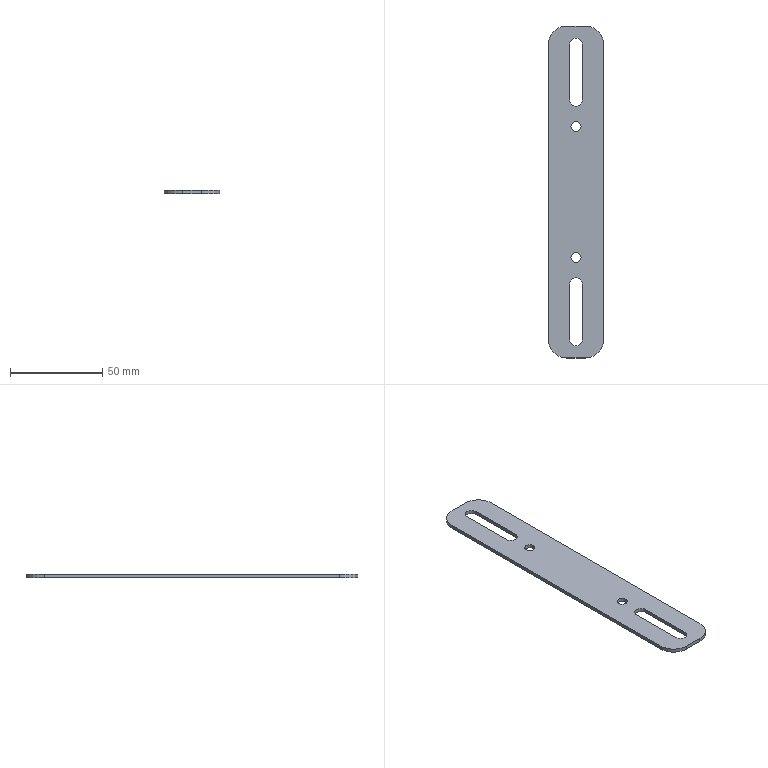Part | SolidWorks | features ICE 2, Extrusion 1, Fillet 1, MirrorPattern 1 | 1 solid | 22 faces | box 30 x 180 x 2 mm | volume 9539 mm3 | cylinder 12 | plane 10 | commonest cylinder face diameters 5.5 x4 7 x4 20 x4
STEP:
#1=CARTESIAN_POINT('',(-2.75,35.5,0.));
#2=VERTEX_POINT('',#1);
#3=CARTESIAN_POINT('',(2.75,35.5,0.));
#4=VERTEX_POINT('',#3);
#5=CARTESIAN_POINT('',(0.,35.5,0.));
#6=DIRECTION('',(0.,0.,1.));
#7=DIRECTION('',(1.,0.,0.));
#8=AXIS2_PLACEMENT_3D('',#5,#6,#7);
#9=CIRCLE('',#8,2.75);
#10=EDGE_CURVE('',#2,#4,#9,.T.);
#11=ORIENTED_EDGE('',*,*,#10,.F.);
#12=CARTESIAN_POINT('',(-2.75,35.5,2.));
#13=VERTEX_POINT('',#12);
#14=CARTESIAN_POINT('',(-2.75,35.5,0.));
#15=DIRECTION('',(0.,0.,1.));
#16=VECTOR('',#15,1000.);
#17=LINE('',#14,#16);
#18=EDGE_CURVE('',#2,#13,#17,.T.);
#19=ORIENTED_EDGE('',*,*,#18,.T.);
#20=CARTESIAN_POINT('',(2.75,35.5,2.));
#21=VERTEX_POINT('',#20);
#22=CARTESIAN_POINT('',(0.,35.5,2.));
#23=DIRECTION('',(0.,0.,1.));
#24=DIRECTION('',(1.,0.,0.));
#25=AXIS2_PLACEMENT_3D('',#22,#23,#24);
#26=CIRCLE('',#25,2.75);
#27=EDGE_CURVE('',#13,#21,#26,.T.);
#28=ORIENTED_EDGE('',*,*,#27,.T.);
#29=CARTESIAN_POINT('',(2.75,35.5,0.));
#30=DIRECTION('',(0.,0.,1.));
#31=VECTOR('',#30,1000.);
#32=LINE('',#29,#31);
#33=EDGE_CURVE('',#4,#21,#32,.T.);
#34=ORIENTED_EDGE('',*,*,#33,.F.);
#35=EDGE_LOOP('',(#11,#19,#28,#34));
#36=FACE_OUTER_BOUND('',#35,.T.);
#37=CARTESIAN_POINT('',(0.,35.5,0.));
#38=DIRECTION('',(0.,0.,1.));
#39=DIRECTION('',(1.,0.,0.));
#40=AXIS2_PLACEMENT_3D('',#37,#38,#39);
#41=CYLINDRICAL_SURFACE('',#40,2.75);
#42=ADVANCED_FACE('',(#36),#41,.F.);
#43=CARTESIAN_POINT('',(-2.75,-35.5,0.));
#44=VERTEX_POINT('',#43);
#45=CARTESIAN_POINT('',(2.75,-35.5,0.));
#46=VERTEX_POINT('',#45);
#47=CARTESIAN_POINT('',(0.,-35.5,0.));
#48=DIRECTION('',(0.,0.,1.));
#49=DIRECTION('',(1.,0.,0.));
#50=AXIS2_PLACEMENT_3D('',#47,#48,#49);
#51=CIRCLE('',#50,2.75);
#52=EDGE_CURVE('',#44,#46,#51,.T.);
#53=ORIENTED_EDGE('',*,*,#52,.F.);
#54=CARTESIAN_POINT('',(-2.75,-35.5,2.));
#55=VERTEX_POINT('',#54);
#56=CARTESIAN_POINT('',(-2.75,-35.5,0.));
#57=DIRECTION('',(0.,0.,1.));
#58=VECTOR('',#57,1000.);
#59=LINE('',#56,#58);
#60=EDGE_CURVE('',#44,#55,#59,.T.);
#61=ORIENTED_EDGE('',*,*,#60,.T.);
#62=CARTESIAN_POINT('',(2.75,-35.5,2.));
#63=VERTEX_POINT('',#62);
#64=CARTESIAN_POINT('',(0.,-35.5,2.));
#65=DIRECTION('',(0.,0.,1.));
#66=DIRECTION('',(1.,0.,0.));
#67=AXIS2_PLACEMENT_3D('',#64,#65,#66);
#68=CIRCLE('',#67,2.75);
#69=EDGE_CURVE('',#55,#63,#68,.T.);
#70=ORIENTED_EDGE('',*,*,#69,.T.);
#71=CARTESIAN_POINT('',(2.75,-35.5,0.));
#72=DIRECTION('',(0.,0.,1.));
#73=VECTOR('',#72,1000.);
#74=LINE('',#71,#73);
#75=EDGE_CURVE('',#46,#63,#74,.T.);
#76=ORIENTED_EDGE('',*,*,#75,.F.);
#77=EDGE_LOOP('',(#53,#61,#70,#76));
#78=FACE_OUTER_BOUND('',#77,.T.);
#79=CARTESIAN_POINT('',(0.,-35.5,0.));
#80=DIRECTION('',(0.,0.,1.));
#81=DIRECTION('',(1.,0.,0.));
#82=AXIS2_PLACEMENT_3D('',#79,#80,#81);
#83=CYLINDRICAL_SURFACE('',#82,2.75);
#84=ADVANCED_FACE('',(#78),#83,.F.);
#85=CARTESIAN_POINT('',(0.,35.5,2.));
#86=DIRECTION('',(0.,0.,1.));
#87=DIRECTION('',(1.,0.,0.));
#88=AXIS2_PLACEMENT_3D('',#85,#86,#87);
#89=CIRCLE('',#88,2.75);
#90=EDGE_CURVE('',#21,#13,#89,.T.);
#91=ORIENTED_EDGE('',*,*,#90,.F.);
#92=ORIENTED_EDGE('',*,*,#27,.F.);
#93=EDGE_LOOP('',(#91,#92));
#94=FACE_BOUND('',#93,.T.);
#95=CARTESIAN_POINT('',(0.,-35.5,2.));
#96=DIRECTION('',(0.,0.,1.));
#97=DIRECTION('',(1.,0.,0.));
#98=AXIS2_PLACEMENT_3D('',#95,#96,#97);
#99=CIRCLE('',#98,2.75);
#100=EDGE_CURVE('',#63,#55,#99,.T.);
#101=ORIENTED_EDGE('',*,*,#100,.F.);
#102=ORIENTED_EDGE('',*,*,#69,.F.);
#103=EDGE_LOOP('',(#101,#102));
#104=FACE_BOUND('',#103,.T.);
#105=CARTESIAN_POINT('',(-5.,-90.,2.));
#106=VERTEX_POINT('',#105);
#107=CARTESIAN_POINT('',(5.,-90.,2.));
#108=VERTEX_POINT('',#107);
#109=CARTESIAN_POINT('',(15.,-90.,2.));
#110=DIRECTION('',(1.,0.,0.));
#111=VECTOR('',#110,1000.);
#112=LINE('',#109,#111);
#113=EDGE_CURVE('',#106,#108,#112,.T.);
#114=ORIENTED_EDGE('',*,*,#113,.T.);
#115=CARTESIAN_POINT('',(15.,-80.,2.));
#116=VERTEX_POINT('',#115);
#117=CARTESIAN_POINT('',(5.,-80.,2.));
#118=DIRECTION('',(0.,0.,1.));
#119=DIRECTION('',(1.,0.,0.));
#120=AXIS2_PLACEMENT_3D('',#117,#118,#119);
#121=CIRCLE('',#120,10.);
#122=EDGE_CURVE('',#108,#116,#121,.T.);
#123=ORIENTED_EDGE('',*,*,#122,.T.);
#124=CARTESIAN_POINT('',(15.,80.,2.));
#125=VERTEX_POINT('',#124);
#126=CARTESIAN_POINT('',(15.,-90.,2.));
#127=DIRECTION('',(0.,1.,0.));
#128=VECTOR('',#127,1000.);
#129=LINE('',#126,#128);
#130=EDGE_CURVE('',#116,#125,#129,.T.);
#131=ORIENTED_EDGE('',*,*,#130,.T.);
#132=CARTESIAN_POINT('',(5.,90.,2.));
#133=VERTEX_POINT('',#132);
#134=CARTESIAN_POINT('',(5.,80.,2.));
#135=DIRECTION('',(0.,0.,1.));
#136=DIRECTION('',(1.,0.,0.));
#137=AXIS2_PLACEMENT_3D('',#134,#135,#136);
#138=CIRCLE('',#137,10.);
#139=EDGE_CURVE('',#125,#133,#138,.T.);
#140=ORIENTED_EDGE('',*,*,#139,.T.);
#141=CARTESIAN_POINT('',(-5.,90.,2.));
#142=VERTEX_POINT('',#141);
#143=CARTESIAN_POINT('',(15.,90.,2.));
#144=DIRECTION('',(-1.,0.,0.));
#145=VECTOR('',#144,1000.);
#146=LINE('',#143,#145);
#147=EDGE_CURVE('',#133,#142,#146,.T.);
#148=ORIENTED_EDGE('',*,*,#147,.T.);
#149=CARTESIAN_POINT('',(-15.,80.,2.));
#150=VERTEX_POINT('',#149);
#151=CARTESIAN_POINT('',(-5.,80.,2.));
#152=DIRECTION('',(0.,0.,1.));
#153=DIRECTION('',(1.,0.,0.));
#154=AXIS2_PLACEMENT_3D('',#151,#152,#153);
#155=CIRCLE('',#154,10.);
#156=EDGE_CURVE('',#142,#150,#155,.T.);
#157=ORIENTED_EDGE('',*,*,#156,.T.);
#158=CARTESIAN_POINT('',(-15.,-80.,2.));
#159=VERTEX_POINT('',#158);
#160=CARTESIAN_POINT('',(-15.,-90.,2.));
#161=DIRECTION('',(0.,-1.,0.));
#162=VECTOR('',#161,1000.);
#163=LINE('',#160,#162);
#164=EDGE_CURVE('',#150,#159,#163,.T.);
#165=ORIENTED_EDGE('',*,*,#164,.T.);
#166=CARTESIAN_POINT('',(-5.,-80.,2.));
#167=DIRECTION('',(0.,0.,1.));
#168=DIRECTION('',(1.,0.,0.));
#169=AXIS2_PLACEMENT_3D('',#166,#167,#168);
#170=CIRCLE('',#169,10.);
#171=EDGE_CURVE('',#159,#106,#170,.T.);
#172=ORIENTED_EDGE('',*,*,#171,.T.);
#173=EDGE_LOOP('',(#114,#123,#131,#140,#148,#157,#165,#172));
#174=FACE_OUTER_BOUND('',#173,.T.);
#175=CARTESIAN_POINT('',(3.5,80.,2.));
#176=VERTEX_POINT('',#175);
#177=CARTESIAN_POINT('',(-3.5,80.,2.));
#178=VERTEX_POINT('',#177);
#179=CARTESIAN_POINT('',(0.,80.,2.));
#180=DIRECTION('',(0.,0.,1.));
#181=DIRECTION('',(1.,0.,0.));
#182=AXIS2_PLACEMENT_3D('',#179,#180,#181);
#183=CIRCLE('',#182,3.5);
#184=EDGE_CURVE('',#176,#178,#183,.T.);
#185=ORIENTED_EDGE('',*,*,#184,.F.);
#186=CARTESIAN_POINT('',(3.5,50.,2.));
#187=VERTEX_POINT('',#186);
#188=CARTESIAN_POINT('',(3.5,80.,2.));
#189=DIRECTION('',(0.,1.,0.));
#190=VECTOR('',#189,1000.);
#191=LINE('',#188,#190);
#192=EDGE_CURVE('',#187,#176,#191,.T.);
#193=ORIENTED_EDGE('',*,*,#192,.F.);
#194=CARTESIAN_POINT('',(-3.5,50.,2.));
#195=VERTEX_POINT('',#194);
#196=CARTESIAN_POINT('',(0.,50.,2.));
#197=DIRECTION('',(0.,0.,1.));
#198=DIRECTION('',(1.,0.,0.));
#199=AXIS2_PLACEMENT_3D('',#196,#197,#198);
#200=CIRCLE('',#199,3.5);
#201=EDGE_CURVE('',#195,#187,#200,.T.);
#202=ORIENTED_EDGE('',*,*,#201,.F.);
#203=CARTESIAN_POINT('',(-3.5,80.,2.));
#204=DIRECTION('',(0.,-1.,0.));
#205=VECTOR('',#204,1000.);
#206=LINE('',#203,#205);
#207=EDGE_CURVE('',#178,#195,#206,.T.);
#208=ORIENTED_EDGE('',*,*,#207,.F.);
#209=EDGE_LOOP('',(#185,#193,#202,#208));
#210=FACE_BOUND('',#209,.T.);
#211=CARTESIAN_POINT('',(3.5,-50.,2.));
#212=VERTEX_POINT('',#211);
#213=CARTESIAN_POINT('',(3.5,-80.,2.));
#214=VERTEX_POINT('',#213);
#215=CARTESIAN_POINT('',(3.5,-80.,2.));
#216=DIRECTION('',(0.,-1.,0.));
#217=VECTOR('',#216,1000.);
#218=LINE('',#215,#217);
#219=EDGE_CURVE('',#212,#214,#218,.T.);
#220=ORIENTED_EDGE('',*,*,#219,.T.);
#221=CARTESIAN_POINT('',(-3.5,-80.,2.));
#222=VERTEX_POINT('',#221);
#223=CARTESIAN_POINT('',(0.,-80.,2.));
#224=DIRECTION('',(0.,0.,-1.));
#225=DIRECTION('',(1.,0.,0.));
#226=AXIS2_PLACEMENT_3D('',#223,#224,#225);
#227=CIRCLE('',#226,3.5);
#228=EDGE_CURVE('',#214,#222,#227,.T.);
#229=ORIENTED_EDGE('',*,*,#228,.T.);
#230=CARTESIAN_POINT('',(-3.5,-50.,2.));
#231=VERTEX_POINT('',#230);
#232=CARTESIAN_POINT('',(-3.5,-80.,2.));
#233=DIRECTION('',(0.,1.,0.));
#234=VECTOR('',#233,1000.);
#235=LINE('',#232,#234);
#236=EDGE_CURVE('',#222,#231,#235,.T.);
#237=ORIENTED_EDGE('',*,*,#236,.T.);
#238=CARTESIAN_POINT('',(0.,-50.,2.));
#239=DIRECTION('',(0.,0.,-1.));
#240=DIRECTION('',(1.,0.,0.));
#241=AXIS2_PLACEMENT_3D('',#238,#239,#240);
#242=CIRCLE('',#241,3.5);
#243=EDGE_CURVE('',#231,#212,#242,.T.);
#244=ORIENTED_EDGE('',*,*,#243,.T.);
#245=EDGE_LOOP('',(#220,#229,#237,#244));
#246=FACE_BOUND('',#245,.T.);
#247=CARTESIAN_POINT('',(0.,0.,2.));
#248=DIRECTION('',(0.,0.,1.));
#249=DIRECTION('',(1.,0.,0.));
#250=AXIS2_PLACEMENT_3D('',#247,#248,#249);
#251=PLANE('',#250);
#252=ADVANCED_FACE('',(#94,#104,#174,#210,#246),#251,.T.);
#253=CARTESIAN_POINT('',(0.,35.5,0.));
#254=DIRECTION('',(0.,0.,1.));
#255=DIRECTION('',(1.,0.,0.));
#256=AXIS2_PLACEMENT_3D('',#253,#254,#255);
#257=CIRCLE('',#256,2.75);
#258=EDGE_CURVE('',#4,#2,#257,.T.);
#259=ORIENTED_EDGE('',*,*,#258,.T.);
#260=ORIENTED_EDGE('',*,*,#10,.T.);
#261=EDGE_LOOP('',(#259,#260));
#262=FACE_BOUND('',#261,.T.);
#263=CARTESIAN_POINT('',(0.,-35.5,0.));
#264=DIRECTION('',(0.,0.,1.));
#265=DIRECTION('',(1.,0.,0.));
#266=AXIS2_PLACEMENT_3D('',#263,#264,#265);
#267=CIRCLE('',#266,2.75);
#268=EDGE_CURVE('',#46,#44,#267,.T.);
#269=ORIENTED_EDGE('',*,*,#268,.T.);
#270=ORIENTED_EDGE('',*,*,#52,.T.);
#271=EDGE_LOOP('',(#269,#270));
#272=FACE_BOUND('',#271,.T.);
#273=CARTESIAN_POINT('',(15.,-80.,0.));
#274=VERTEX_POINT('',#273);
#275=CARTESIAN_POINT('',(15.,80.,0.));
#276=VERTEX_POINT('',#275);
#277=CARTESIAN_POINT('',(15.,-90.,0.));
#278=DIRECTION('',(0.,1.,0.));
#279=VECTOR('',#278,1000.);
#280=LINE('',#277,#279);
#281=EDGE_CURVE('',#274,#276,#280,.T.);
#282=ORIENTED_EDGE('',*,*,#281,.F.);
#283=CARTESIAN_POINT('',(5.,-90.,0.));
#284=VERTEX_POINT('',#283);
#285=CARTESIAN_POINT('',(5.,-80.,0.));
#286=DIRECTION('',(0.,0.,-1.));
#287=DIRECTION('',(1.,0.,0.));
#288=AXIS2_PLACEMENT_3D('',#285,#286,#287);
#289=CIRCLE('',#288,10.);
#290=EDGE_CURVE('',#274,#284,#289,.T.);
#291=ORIENTED_EDGE('',*,*,#290,.T.);
#292=CARTESIAN_POINT('',(-5.,-90.,0.));
#293=VERTEX_POINT('',#292);
#294=CARTESIAN_POINT('',(15.,-90.,0.));
#295=DIRECTION('',(1.,0.,0.));
#296=VECTOR('',#295,1000.);
#297=LINE('',#294,#296);
#298=EDGE_CURVE('',#293,#284,#297,.T.);
#299=ORIENTED_EDGE('',*,*,#298,.F.);
#300=CARTESIAN_POINT('',(-15.,-80.,0.));
#301=VERTEX_POINT('',#300);
#302=CARTESIAN_POINT('',(-5.,-80.,0.));
#303=DIRECTION('',(0.,0.,-1.));
#304=DIRECTION('',(1.,0.,0.));
#305=AXIS2_PLACEMENT_3D('',#302,#303,#304);
#306=CIRCLE('',#305,10.);
#307=EDGE_CURVE('',#293,#301,#306,.T.);
#308=ORIENTED_EDGE('',*,*,#307,.T.);
#309=CARTESIAN_POINT('',(-15.,80.,0.));
#310=VERTEX_POINT('',#309);
#311=CARTESIAN_POINT('',(-15.,-90.,0.));
#312=DIRECTION('',(0.,-1.,0.));
#313=VECTOR('',#312,1000.);
#314=LINE('',#311,#313);
#315=EDGE_CURVE('',#310,#301,#314,.T.);
#316=ORIENTED_EDGE('',*,*,#315,.F.);
#317=CARTESIAN_POINT('',(-5.,90.,0.));
#318=VERTEX_POINT('',#317);
#319=CARTESIAN_POINT('',(-5.,80.,0.));
#320=DIRECTION('',(0.,0.,-1.));
#321=DIRECTION('',(1.,0.,0.));
#322=AXIS2_PLACEMENT_3D('',#319,#320,#321);
#323=CIRCLE('',#322,10.);
#324=EDGE_CURVE('',#310,#318,#323,.T.);
#325=ORIENTED_EDGE('',*,*,#324,.T.);
#326=CARTESIAN_POINT('',(5.,90.,0.));
#327=VERTEX_POINT('',#326);
#328=CARTESIAN_POINT('',(15.,90.,0.));
#329=DIRECTION('',(-1.,0.,0.));
#330=VECTOR('',#329,1000.);
#331=LINE('',#328,#330);
#332=EDGE_CURVE('',#327,#318,#331,.T.);
#333=ORIENTED_EDGE('',*,*,#332,.F.);
#334=CARTESIAN_POINT('',(5.,80.,0.));
#335=DIRECTION('',(0.,0.,-1.));
#336=DIRECTION('',(1.,0.,0.));
#337=AXIS2_PLACEMENT_3D('',#334,#335,#336);
#338=CIRCLE('',#337,10.);
#339=EDGE_CURVE('',#327,#276,#338,.T.);
#340=ORIENTED_EDGE('',*,*,#339,.T.);
#341=EDGE_LOOP('',(#282,#291,#299,#308,#316,#325,#333,#340));
#342=FACE_OUTER_BOUND('',#341,.T.);
#343=CARTESIAN_POINT('',(3.5,50.,0.));
#344=VERTEX_POINT('',#343);
#345=CARTESIAN_POINT('',(3.5,80.,0.));
#346=VERTEX_POINT('',#345);
#347=CARTESIAN_POINT('',(3.5,80.,0.));
#348=DIRECTION('',(0.,1.,0.));
#349=VECTOR('',#348,1000.);
#350=LINE('',#347,#349);
#351=EDGE_CURVE('',#344,#346,#350,.T.);
#352=ORIENTED_EDGE('',*,*,#351,.T.);
#353=CARTESIAN_POINT('',(-3.5,80.,0.));
#354=VERTEX_POINT('',#353);
#355=CARTESIAN_POINT('',(0.,80.,0.));
#356=DIRECTION('',(0.,0.,1.));
#357=DIRECTION('',(1.,0.,0.));
#358=AXIS2_PLACEMENT_3D('',#355,#356,#357);
#359=CIRCLE('',#358,3.5);
#360=EDGE_CURVE('',#346,#354,#359,.T.);
#361=ORIENTED_EDGE('',*,*,#360,.T.);
#362=CARTESIAN_POINT('',(-3.5,50.,0.));
#363=VERTEX_POINT('',#362);
#364=CARTESIAN_POINT('',(-3.5,80.,0.));
#365=DIRECTION('',(0.,-1.,0.));
#366=VECTOR('',#365,1000.);
#367=LINE('',#364,#366);
#368=EDGE_CURVE('',#354,#363,#367,.T.);
#369=ORIENTED_EDGE('',*,*,#368,.T.);
#370=CARTESIAN_POINT('',(0.,50.,0.));
#371=DIRECTION('',(0.,0.,1.));
#372=DIRECTION('',(1.,0.,0.));
#373=AXIS2_PLACEMENT_3D('',#370,#371,#372);
#374=CIRCLE('',#373,3.5);
#375=EDGE_CURVE('',#363,#344,#374,.T.);
#376=ORIENTED_EDGE('',*,*,#375,.T.);
#377=EDGE_LOOP('',(#352,#361,#369,#376));
#378=FACE_BOUND('',#377,.T.);
#379=CARTESIAN_POINT('',(3.5,-80.,0.));
#380=VERTEX_POINT('',#379);
#381=CARTESIAN_POINT('',(-3.5,-80.,0.));
#382=VERTEX_POINT('',#381);
#383=CARTESIAN_POINT('',(0.,-80.,0.));
#384=DIRECTION('',(0.,0.,-1.));
#385=DIRECTION('',(1.,0.,0.));
#386=AXIS2_PLACEMENT_3D('',#383,#384,#385);
#387=CIRCLE('',#386,3.5);
#388=EDGE_CURVE('',#380,#382,#387,.T.);
#389=ORIENTED_EDGE('',*,*,#388,.F.);
#390=CARTESIAN_POINT('',(3.5,-50.,0.));
#391=VERTEX_POINT('',#390);
#392=CARTESIAN_POINT('',(3.5,-80.,0.));
#393=DIRECTION('',(0.,-1.,0.));
#394=VECTOR('',#393,1000.);
#395=LINE('',#392,#394);
#396=EDGE_CURVE('',#391,#380,#395,.T.);
#397=ORIENTED_EDGE('',*,*,#396,.F.);
#398=CARTESIAN_POINT('',(-3.5,-50.,0.));
#399=VERTEX_POINT('',#398);
#400=CARTESIAN_POINT('',(0.,-50.,0.));
#401=DIRECTION('',(0.,0.,-1.));
#402=DIRECTION('',(1.,0.,0.));
#403=AXIS2_PLACEMENT_3D('',#400,#401,#402);
#404=CIRCLE('',#403,3.5);
#405=EDGE_CURVE('',#399,#391,#404,.T.);
#406=ORIENTED_EDGE('',*,*,#405,.F.);
#407=CARTESIAN_POINT('',(-3.5,-80.,0.));
#408=DIRECTION('',(0.,1.,0.));
#409=VECTOR('',#408,1000.);
#410=LINE('',#407,#409);
#411=EDGE_CURVE('',#382,#399,#410,.T.);
#412=ORIENTED_EDGE('',*,*,#411,.F.);
#413=EDGE_LOOP('',(#389,#397,#406,#412));
#414=FACE_BOUND('',#413,.T.);
#415=CARTESIAN_POINT('',(0.,0.,0.));
#416=DIRECTION('',(0.,0.,1.));
#417=DIRECTION('',(1.,0.,0.));
#418=AXIS2_PLACEMENT_3D('',#415,#416,#417);
#419=PLANE('',#418);
#420=ADVANCED_FACE('',(#262,#272,#342,#378,#414),#419,.F.);
#421=ORIENTED_EDGE('',*,*,#315,.T.);
#422=CARTESIAN_POINT('',(-15.,-80.,2.));
#423=DIRECTION('',(0.,0.,1.));
#424=VECTOR('',#423,1000.);
#425=LINE('',#422,#424);
#426=EDGE_CURVE('',#301,#159,#425,.T.);
#427=ORIENTED_EDGE('',*,*,#426,.T.);
#428=ORIENTED_EDGE('',*,*,#164,.F.);
#429=CARTESIAN_POINT('',(-15.,80.,2.));
#430=DIRECTION('',(0.,0.,-1.));
#431=VECTOR('',#430,1000.);
#432=LINE('',#429,#431);
#433=EDGE_CURVE('',#150,#310,#432,.T.);
#434=ORIENTED_EDGE('',*,*,#433,.T.);
#435=EDGE_LOOP('',(#421,#427,#428,#434));
#436=FACE_OUTER_BOUND('',#435,.T.);
#437=CARTESIAN_POINT('',(-15.,-90.,2.));
#438=DIRECTION('',(1.,0.,0.));
#439=DIRECTION('',(0.,0.,-1.));
#440=AXIS2_PLACEMENT_3D('',#437,#438,#439);
#441=PLANE('',#440);
#442=ADVANCED_FACE('',(#436),#441,.F.);
#443=ORIENTED_EDGE('',*,*,#298,.T.);
#444=CARTESIAN_POINT('',(5.,-90.,2.));
#445=DIRECTION('',(0.,0.,1.));
#446=VECTOR('',#445,1000.);
#447=LINE('',#444,#446);
#448=EDGE_CURVE('',#284,#108,#447,.T.);
#449=ORIENTED_EDGE('',*,*,#448,.T.);
#450=ORIENTED_EDGE('',*,*,#113,.F.);
#451=CARTESIAN_POINT('',(-5.,-90.,2.));
#452=DIRECTION('',(0.,0.,-1.));
#453=VECTOR('',#452,1000.);
#454=LINE('',#451,#453);
#455=EDGE_CURVE('',#106,#293,#454,.T.);
#456=ORIENTED_EDGE('',*,*,#455,.T.);
#457=EDGE_LOOP('',(#443,#449,#450,#456));
#458=FACE_OUTER_BOUND('',#457,.T.);
#459=CARTESIAN_POINT('',(15.,-90.,2.));
#460=DIRECTION('',(0.,1.,0.));
#461=DIRECTION('',(0.,0.,1.));
#462=AXIS2_PLACEMENT_3D('',#459,#460,#461);
#463=PLANE('',#462);
#464=ADVANCED_FACE('',(#458),#463,.F.);
#465=ORIENTED_EDGE('',*,*,#130,.F.);
#466=CARTESIAN_POINT('',(15.,-80.,2.));
#467=DIRECTION('',(0.,0.,-1.));
#468=VECTOR('',#467,1000.);
#469=LINE('',#466,#468);
#470=EDGE_CURVE('',#116,#274,#469,.T.);
#471=ORIENTED_EDGE('',*,*,#470,.T.);
#472=ORIENTED_EDGE('',*,*,#281,.T.);
#473=CARTESIAN_POINT('',(15.,80.,2.));
#474=DIRECTION('',(0.,0.,1.));
#475=VECTOR('',#474,1000.);
#476=LINE('',#473,#475);
#477=EDGE_CURVE('',#276,#125,#476,.T.);
#478=ORIENTED_EDGE('',*,*,#477,.T.);
#479=EDGE_LOOP('',(#465,#471,#472,#478));
#480=FACE_OUTER_BOUND('',#479,.T.);
#481=CARTESIAN_POINT('',(15.,-90.,2.));
#482=DIRECTION('',(-1.,0.,0.));
#483=DIRECTION('',(0.,0.,1.));
#484=AXIS2_PLACEMENT_3D('',#481,#482,#483);
#485=PLANE('',#484);
#486=ADVANCED_FACE('',(#480),#485,.F.);
#487=ORIENTED_EDGE('',*,*,#332,.T.);
#488=CARTESIAN_POINT('',(-5.,90.,2.));
#489=DIRECTION('',(0.,0.,1.));
#490=VECTOR('',#489,1000.);
#491=LINE('',#488,#490);
#492=EDGE_CURVE('',#318,#142,#491,.T.);
#493=ORIENTED_EDGE('',*,*,#492,.T.);
#494=ORIENTED_EDGE('',*,*,#147,.F.);
#495=CARTESIAN_POINT('',(5.,90.,2.));
#496=DIRECTION('',(0.,0.,-1.));
#497=VECTOR('',#496,1000.);
#498=LINE('',#495,#497);
#499=EDGE_CURVE('',#133,#327,#498,.T.);
#500=ORIENTED_EDGE('',*,*,#499,.T.);
#501=EDGE_LOOP('',(#487,#493,#494,#500));
#502=FACE_OUTER_BOUND('',#501,.T.);
#503=CARTESIAN_POINT('',(15.,90.,2.));
#504=DIRECTION('',(0.,-1.,0.));
#505=DIRECTION('',(0.,0.,-1.));
#506=AXIS2_PLACEMENT_3D('',#503,#504,#505);
#507=PLANE('',#506);
#508=ADVANCED_FACE('',(#502),#507,.F.);
#509=ORIENTED_EDGE('',*,*,#122,.F.);
#510=ORIENTED_EDGE('',*,*,#448,.F.);
#511=ORIENTED_EDGE('',*,*,#290,.F.);
#512=ORIENTED_EDGE('',*,*,#470,.F.);
#513=EDGE_LOOP('',(#509,#510,#511,#512));
#514=FACE_OUTER_BOUND('',#513,.T.);
#515=CARTESIAN_POINT('',(5.,-80.,2.));
#516=DIRECTION('',(0.,0.,-1.));
#517=DIRECTION('',(-1.,0.,0.));
#518=AXIS2_PLACEMENT_3D('',#515,#516,#517);
#519=CYLINDRICAL_SURFACE('',#518,10.);
#520=ADVANCED_FACE('',(#514),#519,.T.);
#521=ORIENTED_EDGE('',*,*,#171,.F.);
#522=ORIENTED_EDGE('',*,*,#426,.F.);
#523=ORIENTED_EDGE('',*,*,#307,.F.);
#524=ORIENTED_EDGE('',*,*,#455,.F.);
#525=EDGE_LOOP('',(#521,#522,#523,#524));
#526=FACE_OUTER_BOUND('',#525,.T.);
#527=CARTESIAN_POINT('',(-5.,-80.,2.));
#528=DIRECTION('',(0.,0.,-1.));
#529=DIRECTION('',(-1.,0.,0.));
#530=AXIS2_PLACEMENT_3D('',#527,#528,#529);
#531=CYLINDRICAL_SURFACE('',#530,10.);
#532=ADVANCED_FACE('',(#526),#531,.T.);
#533=ORIENTED_EDGE('',*,*,#156,.F.);
#534=ORIENTED_EDGE('',*,*,#492,.F.);
#535=ORIENTED_EDGE('',*,*,#324,.F.);
#536=ORIENTED_EDGE('',*,*,#433,.F.);
#537=EDGE_LOOP('',(#533,#534,#535,#536));
#538=FACE_OUTER_BOUND('',#537,.T.);
#539=CARTESIAN_POINT('',(-5.,80.,2.));
#540=DIRECTION('',(0.,0.,-1.));
#541=DIRECTION('',(-1.,0.,0.));
#542=AXIS2_PLACEMENT_3D('',#539,#540,#541);
#543=CYLINDRICAL_SURFACE('',#542,10.);
#544=ADVANCED_FACE('',(#538),#543,.T.);
#545=ORIENTED_EDGE('',*,*,#139,.F.);
#546=ORIENTED_EDGE('',*,*,#477,.F.);
#547=ORIENTED_EDGE('',*,*,#339,.F.);
#548=ORIENTED_EDGE('',*,*,#499,.F.);
#549=EDGE_LOOP('',(#545,#546,#547,#548));
#550=FACE_OUTER_BOUND('',#549,.T.);
#551=CARTESIAN_POINT('',(5.,80.,2.));
#552=DIRECTION('',(0.,0.,-1.));
#553=DIRECTION('',(-1.,0.,0.));
#554=AXIS2_PLACEMENT_3D('',#551,#552,#553);
#555=CYLINDRICAL_SURFACE('',#554,10.);
#556=ADVANCED_FACE('',(#550),#555,.T.);
#557=ORIENTED_EDGE('',*,*,#184,.T.);
#558=CARTESIAN_POINT('',(-3.5,80.,0.));
#559=DIRECTION('',(0.,0.,1.));
#560=VECTOR('',#559,1000.);
#561=LINE('',#558,#560);
#562=EDGE_CURVE('',#354,#178,#561,.T.);
#563=ORIENTED_EDGE('',*,*,#562,.F.);
#564=ORIENTED_EDGE('',*,*,#360,.F.);
#565=CARTESIAN_POINT('',(3.5,80.,0.));
#566=DIRECTION('',(0.,0.,1.));
#567=VECTOR('',#566,1000.);
#568=LINE('',#565,#567);
#569=EDGE_CURVE('',#346,#176,#568,.T.);
#570=ORIENTED_EDGE('',*,*,#569,.T.);
#571=EDGE_LOOP('',(#557,#563,#564,#570));
#572=FACE_OUTER_BOUND('',#571,.T.);
#573=CARTESIAN_POINT('',(0.,80.,0.));
#574=DIRECTION('',(0.,0.,1.));
#575=DIRECTION('',(1.,0.,0.));
#576=AXIS2_PLACEMENT_3D('',#573,#574,#575);
#577=CYLINDRICAL_SURFACE('',#576,3.5);
#578=ADVANCED_FACE('',(#572),#577,.F.);
#579=ORIENTED_EDGE('',*,*,#192,.T.);
#580=ORIENTED_EDGE('',*,*,#569,.F.);
#581=ORIENTED_EDGE('',*,*,#351,.F.);
#582=CARTESIAN_POINT('',(3.5,50.,0.));
#583=DIRECTION('',(0.,0.,1.));
#584=VECTOR('',#583,1000.);
#585=LINE('',#582,#584);
#586=EDGE_CURVE('',#344,#187,#585,.T.);
#587=ORIENTED_EDGE('',*,*,#586,.T.);
#588=EDGE_LOOP('',(#579,#580,#581,#587));
#589=FACE_OUTER_BOUND('',#588,.T.);
#590=CARTESIAN_POINT('',(3.5,80.,0.));
#591=DIRECTION('',(1.,0.,0.));
#592=DIRECTION('',(0.,1.,0.));
#593=AXIS2_PLACEMENT_3D('',#590,#591,#592);
#594=PLANE('',#593);
#595=ADVANCED_FACE('',(#589),#594,.F.);
#596=ORIENTED_EDGE('',*,*,#201,.T.);
#597=ORIENTED_EDGE('',*,*,#586,.F.);
#598=ORIENTED_EDGE('',*,*,#375,.F.);
#599=CARTESIAN_POINT('',(-3.5,50.,0.));
#600=DIRECTION('',(0.,0.,1.));
#601=VECTOR('',#600,1000.);
#602=LINE('',#599,#601);
#603=EDGE_CURVE('',#363,#195,#602,.T.);
#604=ORIENTED_EDGE('',*,*,#603,.T.);
#605=EDGE_LOOP('',(#596,#597,#598,#604));
#606=FACE_OUTER_BOUND('',#605,.T.);
#607=CARTESIAN_POINT('',(0.,50.,0.));
#608=DIRECTION('',(0.,0.,1.));
#609=DIRECTION('',(1.,0.,0.));
#610=AXIS2_PLACEMENT_3D('',#607,#608,#609);
#611=CYLINDRICAL_SURFACE('',#610,3.5);
#612=ADVANCED_FACE('',(#606),#611,.F.);
#613=ORIENTED_EDGE('',*,*,#207,.T.);
#614=ORIENTED_EDGE('',*,*,#603,.F.);
#615=ORIENTED_EDGE('',*,*,#368,.F.);
#616=ORIENTED_EDGE('',*,*,#562,.T.);
#617=EDGE_LOOP('',(#613,#614,#615,#616));
#618=FACE_OUTER_BOUND('',#617,.T.);
#619=CARTESIAN_POINT('',(-3.5,80.,0.));
#620=DIRECTION('',(-1.,0.,0.));
#621=DIRECTION('',(0.,-1.,0.));
#622=AXIS2_PLACEMENT_3D('',#619,#620,#621);
#623=PLANE('',#622);
#624=ADVANCED_FACE('',(#618),#623,.F.);
#625=ORIENTED_EDGE('',*,*,#228,.F.);
#626=CARTESIAN_POINT('',(3.5,-80.,0.));
#627=DIRECTION('',(0.,0.,1.));
#628=VECTOR('',#627,1000.);
#629=LINE('',#626,#628);
#630=EDGE_CURVE('',#380,#214,#629,.T.);
#631=ORIENTED_EDGE('',*,*,#630,.F.);
#632=ORIENTED_EDGE('',*,*,#388,.T.);
#633=CARTESIAN_POINT('',(-3.5,-80.,0.));
#634=DIRECTION('',(0.,0.,1.));
#635=VECTOR('',#634,1000.);
#636=LINE('',#633,#635);
#637=EDGE_CURVE('',#382,#222,#636,.T.);
#638=ORIENTED_EDGE('',*,*,#637,.T.);
#639=EDGE_LOOP('',(#625,#631,#632,#638));
#640=FACE_OUTER_BOUND('',#639,.T.);
#641=CARTESIAN_POINT('',(0.,-80.,0.));
#642=DIRECTION('',(0.,0.,1.));
#643=DIRECTION('',(1.,0.,0.));
#644=AXIS2_PLACEMENT_3D('',#641,#642,#643);
#645=CYLINDRICAL_SURFACE('',#644,3.5);
#646=ADVANCED_FACE('',(#640),#645,.F.);
#647=ORIENTED_EDGE('',*,*,#236,.F.);
#648=ORIENTED_EDGE('',*,*,#637,.F.);
#649=ORIENTED_EDGE('',*,*,#411,.T.);
#650=CARTESIAN_POINT('',(-3.5,-50.,0.));
#651=DIRECTION('',(0.,0.,1.));
#652=VECTOR('',#651,1000.);
#653=LINE('',#650,#652);
#654=EDGE_CURVE('',#399,#231,#653,.T.);
#655=ORIENTED_EDGE('',*,*,#654,.T.);
#656=EDGE_LOOP('',(#647,#648,#649,#655));
#657=FACE_OUTER_BOUND('',#656,.T.);
#658=CARTESIAN_POINT('',(-3.5,-80.,0.));
#659=DIRECTION('',(1.,0.,0.));
#660=DIRECTION('',(0.,1.,0.));
#661=AXIS2_PLACEMENT_3D('',#658,#659,#660);
#662=PLANE('',#661);
#663=ADVANCED_FACE('',(#657),#662,.T.);
#664=ORIENTED_EDGE('',*,*,#243,.F.);
#665=ORIENTED_EDGE('',*,*,#654,.F.);
#666=ORIENTED_EDGE('',*,*,#405,.T.);
#667=CARTESIAN_POINT('',(3.5,-50.,0.));
#668=DIRECTION('',(0.,0.,1.));
#669=VECTOR('',#668,1000.);
#670=LINE('',#667,#669);
#671=EDGE_CURVE('',#391,#212,#670,.T.);
#672=ORIENTED_EDGE('',*,*,#671,.T.);
#673=EDGE_LOOP('',(#664,#665,#666,#672));
#674=FACE_OUTER_BOUND('',#673,.T.);
#675=CARTESIAN_POINT('',(0.,-50.,0.));
#676=DIRECTION('',(0.,0.,1.));
#677=DIRECTION('',(1.,0.,0.));
#678=AXIS2_PLACEMENT_3D('',#675,#676,#677);
#679=CYLINDRICAL_SURFACE('',#678,3.5);
#680=ADVANCED_FACE('',(#674),#679,.F.);
#681=ORIENTED_EDGE('',*,*,#219,.F.);
#682=ORIENTED_EDGE('',*,*,#671,.F.);
#683=ORIENTED_EDGE('',*,*,#396,.T.);
#684=ORIENTED_EDGE('',*,*,#630,.T.);
#685=EDGE_LOOP('',(#681,#682,#683,#684));
#686=FACE_OUTER_BOUND('',#685,.T.);
#687=CARTESIAN_POINT('',(3.5,-80.,0.));
#688=DIRECTION('',(-1.,0.,0.));
#689=DIRECTION('',(0.,-1.,0.));
#690=AXIS2_PLACEMENT_3D('',#687,#688,#689);
#691=PLANE('',#690);
#692=ADVANCED_FACE('',(#686),#691,.T.);
#693=ORIENTED_EDGE('',*,*,#60,.F.);
#694=ORIENTED_EDGE('',*,*,#268,.F.);
#695=ORIENTED_EDGE('',*,*,#75,.T.);
#696=ORIENTED_EDGE('',*,*,#100,.T.);
#697=EDGE_LOOP('',(#693,#694,#695,#696));
#698=FACE_OUTER_BOUND('',#697,.T.);
#699=CARTESIAN_POINT('',(0.,-35.5,0.));
#700=DIRECTION('',(0.,0.,1.));
#701=DIRECTION('',(1.,0.,0.));
#702=AXIS2_PLACEMENT_3D('',#699,#700,#701);
#703=CYLINDRICAL_SURFACE('',#702,2.75);
#704=ADVANCED_FACE('',(#698),#703,.F.);
#705=ORIENTED_EDGE('',*,*,#18,.F.);
#706=ORIENTED_EDGE('',*,*,#258,.F.);
#707=ORIENTED_EDGE('',*,*,#33,.T.);
#708=ORIENTED_EDGE('',*,*,#90,.T.);
#709=EDGE_LOOP('',(#705,#706,#707,#708));
#710=FACE_OUTER_BOUND('',#709,.T.);
#711=CARTESIAN_POINT('',(0.,35.5,0.));
#712=DIRECTION('',(0.,0.,1.));
#713=DIRECTION('',(1.,0.,0.));
#714=AXIS2_PLACEMENT_3D('',#711,#712,#713);
#715=CYLINDRICAL_SURFACE('',#714,2.75);
#716=ADVANCED_FACE('',(#710),#715,.F.);
#717=CLOSED_SHELL('',(#42,#84,#252,#420,#442,#464,#486,#508,#520,#532,#544,#556,#578,#595,#612,#624,#646,#663,#680,#692,#704,#716));
#718=MANIFOLD_SOLID_BREP('',#717);
#719=CARTESIAN_POINT('',(0.,0.,0.));
#720=DIRECTION('',(0.,0.,1.));
#721=DIRECTION('',(1.,0.,0.));
#722=AXIS2_PLACEMENT_3D('',#719,#720,#721);
#723=(LENGTH_UNIT()NAMED_UNIT(*)SI_UNIT(.MILLI.,.METRE.));
#724=UNCERTAINTY_MEASURE_WITH_UNIT(LENGTH_MEASURE(0.00001),#723,'','');
#725=(NAMED_UNIT(*)PLANE_ANGLE_UNIT()SI_UNIT($,.RADIAN.));
#726=(NAMED_UNIT(*)SI_UNIT($,.STERADIAN.)SOLID_ANGLE_UNIT());
#727=(GEOMETRIC_REPRESENTATION_CONTEXT(3)GLOBAL_UNCERTAINTY_ASSIGNED_CONTEXT((#724))GLOBAL_UNIT_ASSIGNED_CONTEXT((#723,#725,#726))REPRESENTATION_CONTEXT('',''));
#728=ADVANCED_BREP_SHAPE_REPRESENTATION('',(#718,#722),#727);